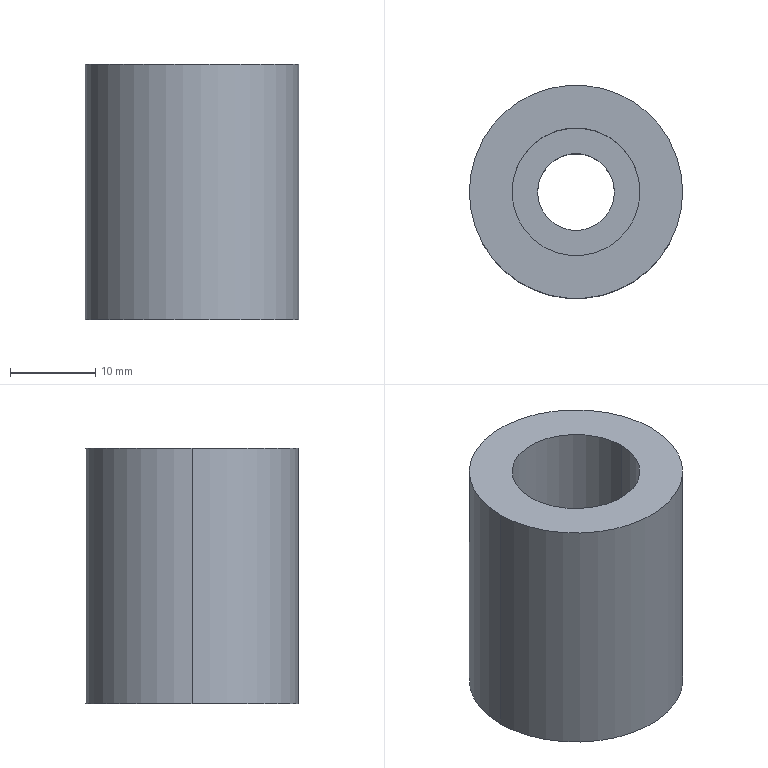Part | STEP file | HXGR200008-05-03 | 1 solid | 9 faces | box 25 x 25 x 30 mm | volume 11121 mm3 | cylinder 6 | plane 3 | commonest cylinder face diameters 9 x2 15 x2 25 x2
STEP:
#1=CARTESIAN_POINT('',(-7.5,0.,15.));
#2=VERTEX_POINT('',#1);
#3=CARTESIAN_POINT('',(7.5,0.,15.));
#4=VERTEX_POINT('',#3);
#5=CARTESIAN_POINT('',(0.,0.,15.));
#6=DIRECTION('',(0.,0.,1.));
#7=DIRECTION('',(1.,0.,0.));
#8=AXIS2_PLACEMENT_3D('',#5,#6,#7);
#9=CIRCLE('',#8,7.5);
#10=EDGE_CURVE('',#2,#4,#9,.T.);
#11=ORIENTED_EDGE('',*,*,#10,.F.);
#12=CARTESIAN_POINT('',(-7.5,0.,30.));
#13=VERTEX_POINT('',#12);
#14=CARTESIAN_POINT('',(-7.5,0.,30.));
#15=DIRECTION('',(0.,0.,1.));
#16=VECTOR('',#15,1000.);
#17=LINE('',#14,#16);
#18=EDGE_CURVE('',#2,#13,#17,.T.);
#19=ORIENTED_EDGE('',*,*,#18,.T.);
#20=CARTESIAN_POINT('',(7.5,0.,30.));
#21=VERTEX_POINT('',#20);
#22=CARTESIAN_POINT('',(0.,0.,30.));
#23=DIRECTION('',(0.,0.,1.));
#24=DIRECTION('',(1.,0.,0.));
#25=AXIS2_PLACEMENT_3D('',#22,#23,#24);
#26=CIRCLE('',#25,7.5);
#27=EDGE_CURVE('',#13,#21,#26,.T.);
#28=ORIENTED_EDGE('',*,*,#27,.T.);
#29=CARTESIAN_POINT('',(7.5,0.,30.));
#30=DIRECTION('',(0.,0.,1.));
#31=VECTOR('',#30,1000.);
#32=LINE('',#29,#31);
#33=EDGE_CURVE('',#4,#21,#32,.T.);
#34=ORIENTED_EDGE('',*,*,#33,.F.);
#35=EDGE_LOOP('',(#11,#19,#28,#34));
#36=FACE_OUTER_BOUND('',#35,.T.);
#37=CARTESIAN_POINT('',(0.,0.,30.));
#38=DIRECTION('',(0.,0.,1.));
#39=DIRECTION('',(1.,0.,0.));
#40=AXIS2_PLACEMENT_3D('',#37,#38,#39);
#41=CYLINDRICAL_SURFACE('',#40,7.5);
#42=ADVANCED_FACE('',(#36),#41,.F.);
#43=CARTESIAN_POINT('',(-4.5,0.,0.));
#44=VERTEX_POINT('',#43);
#45=CARTESIAN_POINT('',(4.5,0.,0.));
#46=VERTEX_POINT('',#45);
#47=CARTESIAN_POINT('',(0.,0.,0.));
#48=DIRECTION('',(0.,0.,1.));
#49=DIRECTION('',(1.,0.,0.));
#50=AXIS2_PLACEMENT_3D('',#47,#48,#49);
#51=CIRCLE('',#50,4.5);
#52=EDGE_CURVE('',#44,#46,#51,.T.);
#53=ORIENTED_EDGE('',*,*,#52,.F.);
#54=CARTESIAN_POINT('',(-4.5,0.,15.));
#55=VERTEX_POINT('',#54);
#56=CARTESIAN_POINT('',(-4.5,0.,30.));
#57=DIRECTION('',(0.,0.,1.));
#58=VECTOR('',#57,1000.);
#59=LINE('',#56,#58);
#60=EDGE_CURVE('',#44,#55,#59,.T.);
#61=ORIENTED_EDGE('',*,*,#60,.T.);
#62=CARTESIAN_POINT('',(4.5,0.,15.));
#63=VERTEX_POINT('',#62);
#64=CARTESIAN_POINT('',(0.,0.,15.));
#65=DIRECTION('',(0.,0.,1.));
#66=DIRECTION('',(1.,0.,0.));
#67=AXIS2_PLACEMENT_3D('',#64,#65,#66);
#68=CIRCLE('',#67,4.5);
#69=EDGE_CURVE('',#55,#63,#68,.T.);
#70=ORIENTED_EDGE('',*,*,#69,.T.);
#71=CARTESIAN_POINT('',(4.5,0.,30.));
#72=DIRECTION('',(0.,0.,1.));
#73=VECTOR('',#72,1000.);
#74=LINE('',#71,#73);
#75=EDGE_CURVE('',#46,#63,#74,.T.);
#76=ORIENTED_EDGE('',*,*,#75,.F.);
#77=EDGE_LOOP('',(#53,#61,#70,#76));
#78=FACE_OUTER_BOUND('',#77,.T.);
#79=CARTESIAN_POINT('',(0.,0.,30.));
#80=DIRECTION('',(0.,0.,1.));
#81=DIRECTION('',(1.,0.,0.));
#82=AXIS2_PLACEMENT_3D('',#79,#80,#81);
#83=CYLINDRICAL_SURFACE('',#82,4.5);
#84=ADVANCED_FACE('',(#78),#83,.F.);
#85=CARTESIAN_POINT('',(12.5,0.,30.));
#86=VERTEX_POINT('',#85);
#87=CARTESIAN_POINT('',(-12.5,0.,30.));
#88=VERTEX_POINT('',#87);
#89=CARTESIAN_POINT('',(0.,0.,30.));
#90=DIRECTION('',(0.,0.,1.));
#91=DIRECTION('',(1.,0.,0.));
#92=AXIS2_PLACEMENT_3D('',#89,#90,#91);
#93=CIRCLE('',#92,12.5);
#94=EDGE_CURVE('',#86,#88,#93,.T.);
#95=ORIENTED_EDGE('',*,*,#94,.F.);
#96=CARTESIAN_POINT('',(12.5,0.,0.));
#97=VERTEX_POINT('',#96);
#98=CARTESIAN_POINT('',(12.5,0.,30.));
#99=DIRECTION('',(0.,0.,-1.));
#100=VECTOR('',#99,1000.);
#101=LINE('',#98,#100);
#102=EDGE_CURVE('',#86,#97,#101,.T.);
#103=ORIENTED_EDGE('',*,*,#102,.T.);
#104=CARTESIAN_POINT('',(-12.5,0.,0.));
#105=VERTEX_POINT('',#104);
#106=CARTESIAN_POINT('',(0.,0.,0.));
#107=DIRECTION('',(0.,0.,1.));
#108=DIRECTION('',(1.,0.,0.));
#109=AXIS2_PLACEMENT_3D('',#106,#107,#108);
#110=CIRCLE('',#109,12.5);
#111=EDGE_CURVE('',#97,#105,#110,.T.);
#112=ORIENTED_EDGE('',*,*,#111,.T.);
#113=CARTESIAN_POINT('',(-12.5,0.,30.));
#114=DIRECTION('',(0.,0.,-1.));
#115=VECTOR('',#114,1000.);
#116=LINE('',#113,#115);
#117=EDGE_CURVE('',#88,#105,#116,.T.);
#118=ORIENTED_EDGE('',*,*,#117,.F.);
#119=EDGE_LOOP('',(#95,#103,#112,#118));
#120=FACE_OUTER_BOUND('',#119,.T.);
#121=CARTESIAN_POINT('',(0.,0.,30.));
#122=DIRECTION('',(0.,0.,-1.));
#123=DIRECTION('',(-1.,0.,0.));
#124=AXIS2_PLACEMENT_3D('',#121,#122,#123);
#125=CYLINDRICAL_SURFACE('',#124,12.5);
#126=ADVANCED_FACE('',(#120),#125,.T.);
#127=ORIENTED_EDGE('',*,*,#102,.F.);
#128=CARTESIAN_POINT('',(0.,0.,30.));
#129=DIRECTION('',(0.,0.,1.));
#130=DIRECTION('',(1.,0.,0.));
#131=AXIS2_PLACEMENT_3D('',#128,#129,#130);
#132=CIRCLE('',#131,12.5);
#133=EDGE_CURVE('',#88,#86,#132,.T.);
#134=ORIENTED_EDGE('',*,*,#133,.F.);
#135=ORIENTED_EDGE('',*,*,#117,.T.);
#136=CARTESIAN_POINT('',(0.,0.,0.));
#137=DIRECTION('',(0.,0.,1.));
#138=DIRECTION('',(1.,0.,0.));
#139=AXIS2_PLACEMENT_3D('',#136,#137,#138);
#140=CIRCLE('',#139,12.5);
#141=EDGE_CURVE('',#105,#97,#140,.T.);
#142=ORIENTED_EDGE('',*,*,#141,.T.);
#143=EDGE_LOOP('',(#127,#134,#135,#142));
#144=FACE_OUTER_BOUND('',#143,.T.);
#145=CARTESIAN_POINT('',(0.,0.,30.));
#146=DIRECTION('',(0.,0.,-1.));
#147=DIRECTION('',(-1.,0.,0.));
#148=AXIS2_PLACEMENT_3D('',#145,#146,#147);
#149=CYLINDRICAL_SURFACE('',#148,12.5);
#150=ADVANCED_FACE('',(#144),#149,.T.);
#151=CARTESIAN_POINT('',(0.,0.,30.));
#152=DIRECTION('',(0.,0.,1.));
#153=DIRECTION('',(1.,0.,0.));
#154=AXIS2_PLACEMENT_3D('',#151,#152,#153);
#155=CIRCLE('',#154,7.5);
#156=EDGE_CURVE('',#21,#13,#155,.T.);
#157=ORIENTED_EDGE('',*,*,#156,.F.);
#158=ORIENTED_EDGE('',*,*,#27,.F.);
#159=EDGE_LOOP('',(#157,#158));
#160=FACE_BOUND('',#159,.T.);
#161=ORIENTED_EDGE('',*,*,#133,.T.);
#162=ORIENTED_EDGE('',*,*,#94,.T.);
#163=EDGE_LOOP('',(#161,#162));
#164=FACE_OUTER_BOUND('',#163,.T.);
#165=CARTESIAN_POINT('',(0.,0.,30.));
#166=DIRECTION('',(0.,0.,1.));
#167=DIRECTION('',(1.,0.,0.));
#168=AXIS2_PLACEMENT_3D('',#165,#166,#167);
#169=PLANE('',#168);
#170=ADVANCED_FACE('',(#160,#164),#169,.T.);
#171=CARTESIAN_POINT('',(0.,0.,0.));
#172=DIRECTION('',(0.,0.,1.));
#173=DIRECTION('',(1.,0.,0.));
#174=AXIS2_PLACEMENT_3D('',#171,#172,#173);
#175=CIRCLE('',#174,4.5);
#176=EDGE_CURVE('',#46,#44,#175,.T.);
#177=ORIENTED_EDGE('',*,*,#176,.T.);
#178=ORIENTED_EDGE('',*,*,#52,.T.);
#179=EDGE_LOOP('',(#177,#178));
#180=FACE_BOUND('',#179,.T.);
#181=ORIENTED_EDGE('',*,*,#141,.F.);
#182=ORIENTED_EDGE('',*,*,#111,.F.);
#183=EDGE_LOOP('',(#181,#182));
#184=FACE_OUTER_BOUND('',#183,.T.);
#185=CARTESIAN_POINT('',(0.,0.,0.));
#186=DIRECTION('',(0.,0.,1.));
#187=DIRECTION('',(1.,0.,0.));
#188=AXIS2_PLACEMENT_3D('',#185,#186,#187);
#189=PLANE('',#188);
#190=ADVANCED_FACE('',(#180,#184),#189,.F.);
#191=ORIENTED_EDGE('',*,*,#60,.F.);
#192=ORIENTED_EDGE('',*,*,#176,.F.);
#193=ORIENTED_EDGE('',*,*,#75,.T.);
#194=CARTESIAN_POINT('',(0.,0.,15.));
#195=DIRECTION('',(0.,0.,1.));
#196=DIRECTION('',(1.,0.,0.));
#197=AXIS2_PLACEMENT_3D('',#194,#195,#196);
#198=CIRCLE('',#197,4.5);
#199=EDGE_CURVE('',#63,#55,#198,.T.);
#200=ORIENTED_EDGE('',*,*,#199,.T.);
#201=EDGE_LOOP('',(#191,#192,#193,#200));
#202=FACE_OUTER_BOUND('',#201,.T.);
#203=CARTESIAN_POINT('',(0.,0.,30.));
#204=DIRECTION('',(0.,0.,1.));
#205=DIRECTION('',(1.,0.,0.));
#206=AXIS2_PLACEMENT_3D('',#203,#204,#205);
#207=CYLINDRICAL_SURFACE('',#206,4.5);
#208=ADVANCED_FACE('',(#202),#207,.F.);
#209=ORIENTED_EDGE('',*,*,#199,.F.);
#210=ORIENTED_EDGE('',*,*,#69,.F.);
#211=EDGE_LOOP('',(#209,#210));
#212=FACE_BOUND('',#211,.T.);
#213=CARTESIAN_POINT('',(0.,0.,15.));
#214=DIRECTION('',(0.,0.,1.));
#215=DIRECTION('',(1.,0.,0.));
#216=AXIS2_PLACEMENT_3D('',#213,#214,#215);
#217=CIRCLE('',#216,7.5);
#218=EDGE_CURVE('',#4,#2,#217,.T.);
#219=ORIENTED_EDGE('',*,*,#218,.T.);
#220=ORIENTED_EDGE('',*,*,#10,.T.);
#221=EDGE_LOOP('',(#219,#220));
#222=FACE_OUTER_BOUND('',#221,.T.);
#223=CARTESIAN_POINT('',(4.5,0.,15.));
#224=DIRECTION('',(0.,0.,-1.));
#225=DIRECTION('',(-1.,0.,0.));
#226=AXIS2_PLACEMENT_3D('',#223,#224,#225);
#227=PLANE('',#226);
#228=ADVANCED_FACE('',(#212,#222),#227,.F.);
#229=ORIENTED_EDGE('',*,*,#18,.F.);
#230=ORIENTED_EDGE('',*,*,#218,.F.);
#231=ORIENTED_EDGE('',*,*,#33,.T.);
#232=ORIENTED_EDGE('',*,*,#156,.T.);
#233=EDGE_LOOP('',(#229,#230,#231,#232));
#234=FACE_OUTER_BOUND('',#233,.T.);
#235=CARTESIAN_POINT('',(0.,0.,30.));
#236=DIRECTION('',(0.,0.,1.));
#237=DIRECTION('',(1.,0.,0.));
#238=AXIS2_PLACEMENT_3D('',#235,#236,#237);
#239=CYLINDRICAL_SURFACE('',#238,7.5);
#240=ADVANCED_FACE('',(#234),#239,.F.);
#241=CLOSED_SHELL('',(#42,#84,#126,#150,#170,#190,#208,#228,#240));
#242=MANIFOLD_SOLID_BREP('',#241);
#243=CARTESIAN_POINT('',(0.,0.,0.));
#244=DIRECTION('',(0.,0.,1.));
#245=DIRECTION('',(1.,0.,0.));
#246=AXIS2_PLACEMENT_3D('',#243,#244,#245);
#247=(LENGTH_UNIT()NAMED_UNIT(*)SI_UNIT(.MILLI.,.METRE.));
#248=UNCERTAINTY_MEASURE_WITH_UNIT(LENGTH_MEASURE(0.00001),#247,'','');
#249=(NAMED_UNIT(*)PLANE_ANGLE_UNIT()SI_UNIT($,.RADIAN.));
#250=(NAMED_UNIT(*)SI_UNIT($,.STERADIAN.)SOLID_ANGLE_UNIT());
#251=(GEOMETRIC_REPRESENTATION_CONTEXT(3)GLOBAL_UNCERTAINTY_ASSIGNED_CONTEXT((#248))GLOBAL_UNIT_ASSIGNED_CONTEXT((#247,#249,#250))REPRESENTATION_CONTEXT('',''));
#252=ADVANCED_BREP_SHAPE_REPRESENTATION('',(#242,#246),#251);